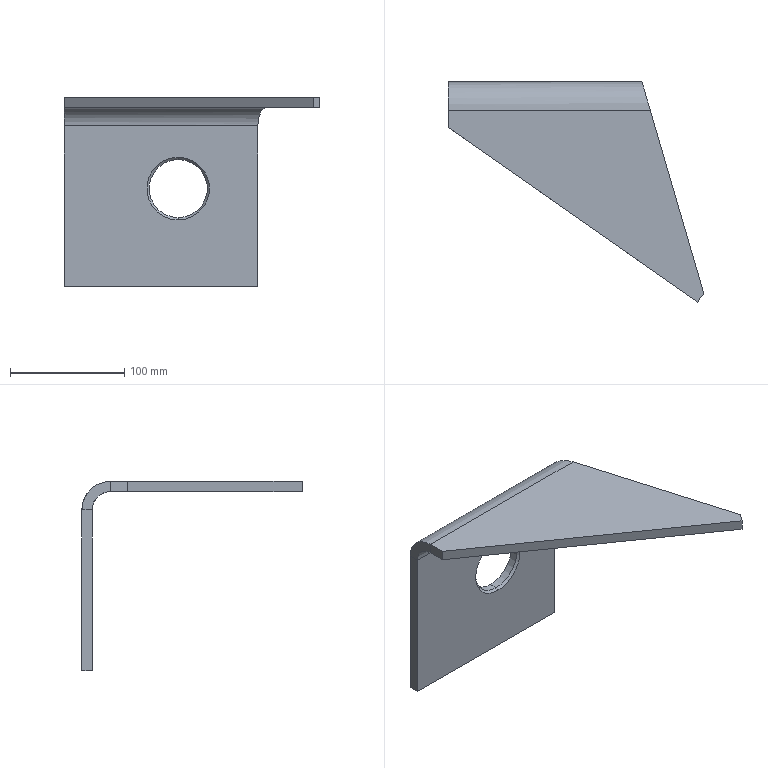Part | SolidWorks | features ICE 2, Chamfer 1, FlatPattern 1, SMBaseFlange 1, SheetMetal 1 | 1 solid | 19 faces | box 224.289 x 193.117 x 166 mm | volume 401605 mm3 | plane 12 | cylinder 4 | cone 2 | spline 1 | commonest cylinder face diameters 51 x2 32 x1 50 x1
STEP:
#1=CARTESIAN_POINT('',(100.,-7.,111.5));
#2=VERTEX_POINT('',#1);
#3=CARTESIAN_POINT('',(100.,-7.,60.5));
#4=VERTEX_POINT('',#3);
#5=CARTESIAN_POINT('',(100.,-7.,86.));
#6=DIRECTION('',(0.,-1.,0.));
#7=DIRECTION('',(0.,0.,-1.));
#8=AXIS2_PLACEMENT_3D('',#5,#6,#7);
#9=CIRCLE('',#8,25.5);
#10=EDGE_CURVE('',#2,#4,#9,.T.);
#11=ORIENTED_EDGE('',*,*,#10,.F.);
#12=CARTESIAN_POINT('',(100.,-9.,113.5));
#13=VERTEX_POINT('',#12);
#14=CARTESIAN_POINT('',(100.,-7.,111.5));
#15=DIRECTION('',(0.,-0.7071,0.7071));
#16=VECTOR('',#15,1000.);
#17=LINE('',#14,#16);
#18=EDGE_CURVE('',#2,#13,#17,.T.);
#19=ORIENTED_EDGE('',*,*,#18,.T.);
#20=CARTESIAN_POINT('',(100.,-9.,58.5));
#21=VERTEX_POINT('',#20);
#22=CARTESIAN_POINT('',(100.,-9.,86.));
#23=DIRECTION('',(0.,1.,0.));
#24=DIRECTION('',(0.,0.,-1.));
#25=AXIS2_PLACEMENT_3D('',#22,#23,#24);
#26=CIRCLE('',#25,27.5);
#27=EDGE_CURVE('',#21,#13,#26,.T.);
#28=ORIENTED_EDGE('',*,*,#27,.F.);
#29=CARTESIAN_POINT('',(100.,-7.,60.5));
#30=DIRECTION('',(0.,-0.7071,-0.7071));
#31=VECTOR('',#30,1000.);
#32=LINE('',#29,#31);
#33=EDGE_CURVE('',#4,#21,#32,.T.);
#34=ORIENTED_EDGE('',*,*,#33,.F.);
#35=EDGE_LOOP('',(#11,#19,#28,#34));
#36=FACE_OUTER_BOUND('',#35,.T.);
#37=CARTESIAN_POINT('',(100.,-7.,86.));
#38=DIRECTION('',(0.,-1.,0.));
#39=DIRECTION('',(0.,0.,-1.));
#40=AXIS2_PLACEMENT_3D('',#37,#38,#39);
#41=CONICAL_SURFACE('',#40,25.5,0.7854);
#42=ADVANCED_FACE('',(#36),#41,.F.);
#43=ORIENTED_EDGE('',*,*,#10,.T.);
#44=CARTESIAN_POINT('',(100.,0.,60.5));
#45=VERTEX_POINT('',#44);
#46=CARTESIAN_POINT('',(100.,-193.117,60.5));
#47=DIRECTION('',(0.,1.,0.));
#48=VECTOR('',#47,1000.);
#49=LINE('',#46,#48);
#50=EDGE_CURVE('',#4,#45,#49,.T.);
#51=ORIENTED_EDGE('',*,*,#50,.T.);
#52=CARTESIAN_POINT('',(100.,0.,111.5));
#53=VERTEX_POINT('',#52);
#54=CARTESIAN_POINT('',(100.,0.,86.));
#55=DIRECTION('',(0.,1.,0.));
#56=DIRECTION('',(0.,0.,1.));
#57=AXIS2_PLACEMENT_3D('',#54,#55,#56);
#58=CIRCLE('',#57,25.5);
#59=EDGE_CURVE('',#45,#53,#58,.T.);
#60=ORIENTED_EDGE('',*,*,#59,.T.);
#61=CARTESIAN_POINT('',(100.,-193.117,111.5));
#62=DIRECTION('',(0.,1.,0.));
#63=VECTOR('',#62,1000.);
#64=LINE('',#61,#63);
#65=EDGE_CURVE('',#2,#53,#64,.T.);
#66=ORIENTED_EDGE('',*,*,#65,.F.);
#67=EDGE_LOOP('',(#43,#51,#60,#66));
#68=FACE_OUTER_BOUND('',#67,.T.);
#69=CARTESIAN_POINT('',(100.,-193.117,86.));
#70=DIRECTION('',(0.,1.,0.));
#71=DIRECTION('',(0.,0.,1.));
#72=AXIS2_PLACEMENT_3D('',#69,#70,#71);
#73=CYLINDRICAL_SURFACE('',#72,25.5);
#74=ADVANCED_FACE('',(#68),#73,.F.);
#75=CARTESIAN_POINT('',(0.,-25.,157.));
#76=VERTEX_POINT('',#75);
#77=CARTESIAN_POINT('',(0.,-40.,157.));
#78=VERTEX_POINT('',#77);
#79=CARTESIAN_POINT('',(0.,0.,157.));
#80=DIRECTION('',(0.,-1.,0.));
#81=VECTOR('',#80,1000.);
#82=LINE('',#79,#81);
#83=EDGE_CURVE('',#76,#78,#82,.T.);
#84=ORIENTED_EDGE('',*,*,#83,.T.);
#85=CARTESIAN_POINT('',(0.,-40.,166.));
#86=VERTEX_POINT('',#85);
#87=CARTESIAN_POINT('',(0.,-40.,157.));
#88=DIRECTION('',(0.,0.,1.));
#89=VECTOR('',#88,1000.);
#90=LINE('',#87,#89);
#91=EDGE_CURVE('',#78,#86,#90,.T.);
#92=ORIENTED_EDGE('',*,*,#91,.T.);
#93=CARTESIAN_POINT('',(0.,-25.,166.));
#94=VERTEX_POINT('',#93);
#95=CARTESIAN_POINT('',(0.,0.,166.));
#96=DIRECTION('',(0.,-1.,0.));
#97=VECTOR('',#96,1000.);
#98=LINE('',#95,#97);
#99=EDGE_CURVE('',#94,#86,#98,.T.);
#100=ORIENTED_EDGE('',*,*,#99,.F.);
#101=CARTESIAN_POINT('',(0.,-25.,166.));
#102=DIRECTION('',(0.,0.,-1.));
#103=VECTOR('',#102,1000.);
#104=LINE('',#101,#103);
#105=EDGE_CURVE('',#94,#76,#104,.T.);
#106=ORIENTED_EDGE('',*,*,#105,.T.);
#107=EDGE_LOOP('',(#84,#92,#100,#106));
#108=FACE_OUTER_BOUND('',#107,.T.);
#109=CARTESIAN_POINT('',(0.,-9.,141.));
#110=DIRECTION('',(-1.,0.,0.));
#111=DIRECTION('',(0.,0.,1.));
#112=AXIS2_PLACEMENT_3D('',#109,#110,#111);
#113=PLANE('',#112);
#114=ADVANCED_FACE('',(#108),#113,.T.);
#115=CARTESIAN_POINT('',(218.67,-193.117,166.));
#116=VERTEX_POINT('',#115);
#117=CARTESIAN_POINT('',(134.53,-134.201,166.));
#118=DIRECTION('',(0.8191,-0.5736,0.));
#119=VECTOR('',#118,1000.);
#120=LINE('',#117,#119);
#121=EDGE_CURVE('',#86,#116,#120,.T.);
#122=ORIENTED_EDGE('',*,*,#121,.T.);
#123=CARTESIAN_POINT('',(224.289,-185.603,166.));
#124=VERTEX_POINT('',#123);
#125=CARTESIAN_POINT('',(314.815,-64.545,166.));
#126=DIRECTION('',(0.5989,0.8008,0.));
#127=VECTOR('',#126,1000.);
#128=LINE('',#125,#127);
#129=EDGE_CURVE('',#116,#124,#128,.T.);
#130=ORIENTED_EDGE('',*,*,#129,.T.);
#131=CARTESIAN_POINT('',(177.312,-25.,166.));
#132=VERTEX_POINT('',#131);
#133=CARTESIAN_POINT('',(174.611,-15.763,166.));
#134=DIRECTION('',(-0.2807,0.9598,0.));
#135=VECTOR('',#134,1000.);
#136=LINE('',#133,#135);
#137=EDGE_CURVE('',#124,#132,#136,.T.);
#138=ORIENTED_EDGE('',*,*,#137,.T.);
#139=CARTESIAN_POINT('',(228.5,-25.,166.));
#140=DIRECTION('',(-1.,0.,0.));
#141=VECTOR('',#140,1000.);
#142=LINE('',#139,#141);
#143=EDGE_CURVE('',#132,#94,#142,.T.);
#144=ORIENTED_EDGE('',*,*,#143,.T.);
#145=ORIENTED_EDGE('',*,*,#99,.T.);
#146=EDGE_LOOP('',(#122,#130,#138,#144,#145));
#147=FACE_OUTER_BOUND('',#146,.T.);
#148=CARTESIAN_POINT('',(228.5,0.,166.));
#149=DIRECTION('',(0.,0.,-1.));
#150=DIRECTION('',(-1.,0.,0.));
#151=AXIS2_PLACEMENT_3D('',#148,#149,#150);
#152=PLANE('',#151);
#153=ADVANCED_FACE('',(#147),#152,.F.);
#154=CARTESIAN_POINT('',(218.67,-193.117,157.));
#155=VERTEX_POINT('',#154);
#156=CARTESIAN_POINT('',(224.289,-185.603,157.));
#157=VERTEX_POINT('',#156);
#158=CARTESIAN_POINT('',(314.815,-64.545,157.));
#159=DIRECTION('',(0.5989,0.8008,0.));
#160=VECTOR('',#159,1000.);
#161=LINE('',#158,#160);
#162=EDGE_CURVE('',#155,#157,#161,.T.);
#163=ORIENTED_EDGE('',*,*,#162,.F.);
#164=CARTESIAN_POINT('',(134.53,-134.201,157.));
#165=DIRECTION('',(0.8191,-0.5736,0.));
#166=VECTOR('',#165,1000.);
#167=LINE('',#164,#166);
#168=EDGE_CURVE('',#78,#155,#167,.T.);
#169=ORIENTED_EDGE('',*,*,#168,.F.);
#170=ORIENTED_EDGE('',*,*,#83,.F.);
#171=CARTESIAN_POINT('',(177.312,-25.,157.));
#172=VERTEX_POINT('',#171);
#173=CARTESIAN_POINT('',(228.5,-25.,157.));
#174=DIRECTION('',(-1.,0.,0.));
#175=VECTOR('',#174,1000.);
#176=LINE('',#173,#175);
#177=EDGE_CURVE('',#172,#76,#176,.T.);
#178=ORIENTED_EDGE('',*,*,#177,.F.);
#179=CARTESIAN_POINT('',(174.611,-15.763,157.));
#180=DIRECTION('',(-0.2807,0.9598,0.));
#181=VECTOR('',#180,1000.);
#182=LINE('',#179,#181);
#183=EDGE_CURVE('',#157,#172,#182,.T.);
#184=ORIENTED_EDGE('',*,*,#183,.F.);
#185=EDGE_LOOP('',(#163,#169,#170,#178,#184));
#186=FACE_OUTER_BOUND('',#185,.T.);
#187=CARTESIAN_POINT('',(228.5,0.,157.));
#188=DIRECTION('',(0.,0.,-1.));
#189=DIRECTION('',(-1.,0.,0.));
#190=AXIS2_PLACEMENT_3D('',#187,#188,#189);
#191=PLANE('',#190);
#192=ADVANCED_FACE('',(#186),#191,.T.);
#193=CARTESIAN_POINT('',(170.,-9.,141.));
#194=VERTEX_POINT('',#193);
#195=CARTESIAN_POINT('',(0.,-9.,141.));
#196=VERTEX_POINT('',#195);
#197=CARTESIAN_POINT('',(228.5,-9.,141.));
#198=DIRECTION('',(-1.,0.,0.));
#199=VECTOR('',#198,1000.);
#200=LINE('',#197,#199);
#201=EDGE_CURVE('',#194,#196,#200,.T.);
#202=ORIENTED_EDGE('',*,*,#201,.F.);
#203=CARTESIAN_POINT('',(177.312,-25.,157.));
#204=CARTESIAN_POINT('',(173.029,-15.627,157.));
#205=CARTESIAN_POINT('',(170.,-9.,150.373));
#206=CARTESIAN_POINT('',(170.,-9.,141.));
#207=(BOUNDED_CURVE()B_SPLINE_CURVE(3,(#203,#204,#205,#206),.UNSPECIFIED.,.F.,.T.)B_SPLINE_CURVE_WITH_KNOTS((4,4),(4.712,6.283),.UNSPECIFIED.)CURVE()GEOMETRIC_REPRESENTATION_ITEM()RATIONAL_B_SPLINE_CURVE((1.,0.8047,0.8047,1.))REPRESENTATION_ITEM(''));
#208=EDGE_CURVE('',#172,#194,#207,.T.);
#209=ORIENTED_EDGE('',*,*,#208,.F.);
#210=ORIENTED_EDGE('',*,*,#177,.T.);
#211=CARTESIAN_POINT('',(0.,-25.,141.));
#212=DIRECTION('',(1.,0.,0.));
#213=DIRECTION('',(0.,0.,-1.));
#214=AXIS2_PLACEMENT_3D('',#211,#212,#213);
#215=CIRCLE('',#214,16.);
#216=EDGE_CURVE('',#196,#76,#215,.T.);
#217=ORIENTED_EDGE('',*,*,#216,.F.);
#218=EDGE_LOOP('',(#202,#209,#210,#217));
#219=FACE_OUTER_BOUND('',#218,.T.);
#220=CARTESIAN_POINT('',(228.5,-25.,141.));
#221=DIRECTION('',(-1.,0.,0.));
#222=DIRECTION('',(0.,0.,1.));
#223=AXIS2_PLACEMENT_3D('',#220,#221,#222);
#224=CYLINDRICAL_SURFACE('',#223,16.);
#225=ADVANCED_FACE('',(#219),#224,.F.);
#226=ORIENTED_EDGE('',*,*,#27,.T.);
#227=CARTESIAN_POINT('',(100.,-9.,86.));
#228=DIRECTION('',(0.,1.,0.));
#229=DIRECTION('',(0.,0.,-1.));
#230=AXIS2_PLACEMENT_3D('',#227,#228,#229);
#231=CIRCLE('',#230,27.5);
#232=EDGE_CURVE('',#13,#21,#231,.T.);
#233=ORIENTED_EDGE('',*,*,#232,.T.);
#234=EDGE_LOOP('',(#226,#233));
#235=FACE_BOUND('',#234,.T.);
#236=CARTESIAN_POINT('',(170.,-9.,0.));
#237=VERTEX_POINT('',#236);
#238=CARTESIAN_POINT('',(0.,-9.,0.));
#239=VERTEX_POINT('',#238);
#240=CARTESIAN_POINT('',(228.5,-9.,0.));
#241=DIRECTION('',(-1.,0.,0.));
#242=VECTOR('',#241,1000.);
#243=LINE('',#240,#242);
#244=EDGE_CURVE('',#237,#239,#243,.T.);
#245=ORIENTED_EDGE('',*,*,#244,.F.);
#246=CARTESIAN_POINT('',(170.,-9.,0.));
#247=DIRECTION('',(0.,0.,1.));
#248=VECTOR('',#247,1000.);
#249=LINE('',#246,#248);
#250=EDGE_CURVE('',#237,#194,#249,.T.);
#251=ORIENTED_EDGE('',*,*,#250,.T.);
#252=ORIENTED_EDGE('',*,*,#201,.T.);
#253=CARTESIAN_POINT('',(0.,-9.,0.));
#254=DIRECTION('',(0.,0.,1.));
#255=VECTOR('',#254,1000.);
#256=LINE('',#253,#255);
#257=EDGE_CURVE('',#239,#196,#256,.T.);
#258=ORIENTED_EDGE('',*,*,#257,.F.);
#259=EDGE_LOOP('',(#245,#251,#252,#258));
#260=FACE_OUTER_BOUND('',#259,.T.);
#261=CARTESIAN_POINT('',(228.5,-9.,0.));
#262=DIRECTION('',(0.,-1.,0.));
#263=DIRECTION('',(0.,0.,-1.));
#264=AXIS2_PLACEMENT_3D('',#261,#262,#263);
#265=PLANE('',#264);
#266=ADVANCED_FACE('',(#235,#260),#265,.T.);
#267=CARTESIAN_POINT('',(170.,0.,0.));
#268=VERTEX_POINT('',#267);
#269=CARTESIAN_POINT('',(0.,0.,0.));
#270=VERTEX_POINT('',#269);
#271=CARTESIAN_POINT('',(228.5,0.,0.));
#272=DIRECTION('',(-1.,0.,0.));
#273=VECTOR('',#272,1000.);
#274=LINE('',#271,#273);
#275=EDGE_CURVE('',#268,#270,#274,.T.);
#276=ORIENTED_EDGE('',*,*,#275,.F.);
#277=CARTESIAN_POINT('',(170.,0.,0.));
#278=DIRECTION('',(0.,-1.,0.));
#279=VECTOR('',#278,1000.);
#280=LINE('',#277,#279);
#281=EDGE_CURVE('',#268,#237,#280,.T.);
#282=ORIENTED_EDGE('',*,*,#281,.T.);
#283=ORIENTED_EDGE('',*,*,#244,.T.);
#284=CARTESIAN_POINT('',(0.,0.,0.));
#285=DIRECTION('',(0.,-1.,0.));
#286=VECTOR('',#285,1000.);
#287=LINE('',#284,#286);
#288=EDGE_CURVE('',#270,#239,#287,.T.);
#289=ORIENTED_EDGE('',*,*,#288,.F.);
#290=EDGE_LOOP('',(#276,#282,#283,#289));
#291=FACE_OUTER_BOUND('',#290,.T.);
#292=CARTESIAN_POINT('',(228.5,0.,0.));
#293=DIRECTION('',(0.,0.,-1.));
#294=DIRECTION('',(-1.,0.,0.));
#295=AXIS2_PLACEMENT_3D('',#292,#293,#294);
#296=PLANE('',#295);
#297=ADVANCED_FACE('',(#291),#296,.T.);
#298=CARTESIAN_POINT('',(100.,0.,86.));
#299=DIRECTION('',(0.,1.,0.));
#300=DIRECTION('',(0.,0.,1.));
#301=AXIS2_PLACEMENT_3D('',#298,#299,#300);
#302=CIRCLE('',#301,25.5);
#303=EDGE_CURVE('',#53,#45,#302,.T.);
#304=ORIENTED_EDGE('',*,*,#303,.F.);
#305=ORIENTED_EDGE('',*,*,#59,.F.);
#306=EDGE_LOOP('',(#304,#305));
#307=FACE_BOUND('',#306,.T.);
#308=CARTESIAN_POINT('',(170.,0.,141.));
#309=VERTEX_POINT('',#308);
#310=CARTESIAN_POINT('',(170.,0.,0.));
#311=DIRECTION('',(0.,0.,1.));
#312=VECTOR('',#311,1000.);
#313=LINE('',#310,#312);
#314=EDGE_CURVE('',#268,#309,#313,.T.);
#315=ORIENTED_EDGE('',*,*,#314,.F.);
#316=ORIENTED_EDGE('',*,*,#275,.T.);
#317=CARTESIAN_POINT('',(0.,0.,141.));
#318=VERTEX_POINT('',#317);
#319=CARTESIAN_POINT('',(0.,0.,0.));
#320=DIRECTION('',(0.,0.,1.));
#321=VECTOR('',#320,1000.);
#322=LINE('',#319,#321);
#323=EDGE_CURVE('',#270,#318,#322,.T.);
#324=ORIENTED_EDGE('',*,*,#323,.T.);
#325=CARTESIAN_POINT('',(228.5,0.,141.));
#326=DIRECTION('',(-1.,0.,0.));
#327=VECTOR('',#326,1000.);
#328=LINE('',#325,#327);
#329=EDGE_CURVE('',#309,#318,#328,.T.);
#330=ORIENTED_EDGE('',*,*,#329,.F.);
#331=EDGE_LOOP('',(#315,#316,#324,#330));
#332=FACE_OUTER_BOUND('',#331,.T.);
#333=CARTESIAN_POINT('',(228.5,0.,0.));
#334=DIRECTION('',(0.,-1.,0.));
#335=DIRECTION('',(0.,0.,-1.));
#336=AXIS2_PLACEMENT_3D('',#333,#334,#335);
#337=PLANE('',#336);
#338=ADVANCED_FACE('',(#307,#332),#337,.F.);
#339=CARTESIAN_POINT('',(177.312,-25.,166.));
#340=CARTESIAN_POINT('',(173.029,-10.355,166.));
#341=CARTESIAN_POINT('',(170.,0.,155.645));
#342=CARTESIAN_POINT('',(170.,0.,141.));
#343=(BOUNDED_CURVE()B_SPLINE_CURVE(3,(#339,#340,#341,#342),.UNSPECIFIED.,.F.,.T.)B_SPLINE_CURVE_WITH_KNOTS((4,4),(4.712,6.283),.UNSPECIFIED.)CURVE()GEOMETRIC_REPRESENTATION_ITEM()RATIONAL_B_SPLINE_CURVE((1.,0.8047,0.8047,1.))REPRESENTATION_ITEM(''));
#344=EDGE_CURVE('',#132,#309,#343,.T.);
#345=ORIENTED_EDGE('',*,*,#344,.T.);
#346=ORIENTED_EDGE('',*,*,#329,.T.);
#347=CARTESIAN_POINT('',(0.,-25.,141.));
#348=DIRECTION('',(1.,0.,0.));
#349=DIRECTION('',(0.,0.,1.));
#350=AXIS2_PLACEMENT_3D('',#347,#348,#349);
#351=CIRCLE('',#350,25.);
#352=EDGE_CURVE('',#318,#94,#351,.T.);
#353=ORIENTED_EDGE('',*,*,#352,.T.);
#354=ORIENTED_EDGE('',*,*,#143,.F.);
#355=EDGE_LOOP('',(#345,#346,#353,#354));
#356=FACE_OUTER_BOUND('',#355,.T.);
#357=CARTESIAN_POINT('',(228.5,-25.,141.));
#358=DIRECTION('',(-1.,0.,0.));
#359=DIRECTION('',(0.,0.,1.));
#360=AXIS2_PLACEMENT_3D('',#357,#358,#359);
#361=CYLINDRICAL_SURFACE('',#360,25.);
#362=ADVANCED_FACE('',(#356),#361,.T.);
#363=ORIENTED_EDGE('',*,*,#105,.F.);
#364=ORIENTED_EDGE('',*,*,#352,.F.);
#365=CARTESIAN_POINT('',(0.,-9.,141.));
#366=DIRECTION('',(0.,1.,0.));
#367=VECTOR('',#366,1000.);
#368=LINE('',#365,#367);
#369=EDGE_CURVE('',#196,#318,#368,.T.);
#370=ORIENTED_EDGE('',*,*,#369,.F.);
#371=ORIENTED_EDGE('',*,*,#216,.T.);
#372=EDGE_LOOP('',(#363,#364,#370,#371));
#373=FACE_OUTER_BOUND('',#372,.T.);
#374=CARTESIAN_POINT('',(0.,-25.,166.));
#375=DIRECTION('',(-1.,0.,0.));
#376=DIRECTION('',(0.,0.,1.));
#377=AXIS2_PLACEMENT_3D('',#374,#375,#376);
#378=PLANE('',#377);
#379=ADVANCED_FACE('',(#373),#378,.T.);
#380=ORIENTED_EDGE('',*,*,#257,.T.);
#381=ORIENTED_EDGE('',*,*,#369,.T.);
#382=ORIENTED_EDGE('',*,*,#323,.F.);
#383=ORIENTED_EDGE('',*,*,#288,.T.);
#384=EDGE_LOOP('',(#380,#381,#382,#383));
#385=FACE_OUTER_BOUND('',#384,.T.);
#386=CARTESIAN_POINT('',(0.,-25.,141.));
#387=DIRECTION('',(1.,0.,0.));
#388=DIRECTION('',(0.,0.,-1.));
#389=AXIS2_PLACEMENT_3D('',#386,#387,#388);
#390=PLANE('',#389);
#391=ADVANCED_FACE('',(#385),#390,.F.);
#392=ORIENTED_EDGE('',*,*,#91,.F.);
#393=ORIENTED_EDGE('',*,*,#168,.T.);
#394=CARTESIAN_POINT('',(218.67,-193.117,157.));
#395=DIRECTION('',(0.,0.,1.));
#396=VECTOR('',#395,1000.);
#397=LINE('',#394,#396);
#398=EDGE_CURVE('',#155,#116,#397,.T.);
#399=ORIENTED_EDGE('',*,*,#398,.T.);
#400=ORIENTED_EDGE('',*,*,#121,.F.);
#401=EDGE_LOOP('',(#392,#393,#399,#400));
#402=FACE_OUTER_BOUND('',#401,.T.);
#403=CARTESIAN_POINT('',(134.53,-134.201,157.));
#404=DIRECTION('',(0.5736,0.8191,0.));
#405=DIRECTION('',(0.8191,-0.5736,0.));
#406=AXIS2_PLACEMENT_3D('',#403,#404,#405);
#407=PLANE('',#406);
#408=ADVANCED_FACE('',(#402),#407,.F.);
#409=ORIENTED_EDGE('',*,*,#398,.F.);
#410=ORIENTED_EDGE('',*,*,#162,.T.);
#411=CARTESIAN_POINT('',(224.289,-185.603,157.));
#412=DIRECTION('',(0.,0.,1.));
#413=VECTOR('',#412,1000.);
#414=LINE('',#411,#413);
#415=EDGE_CURVE('',#157,#124,#414,.T.);
#416=ORIENTED_EDGE('',*,*,#415,.T.);
#417=ORIENTED_EDGE('',*,*,#129,.F.);
#418=EDGE_LOOP('',(#409,#410,#416,#417));
#419=FACE_OUTER_BOUND('',#418,.T.);
#420=CARTESIAN_POINT('',(314.815,-64.545,157.));
#421=DIRECTION('',(-0.8008,0.5989,0.));
#422=DIRECTION('',(0.5989,0.8008,0.));
#423=AXIS2_PLACEMENT_3D('',#420,#421,#422);
#424=PLANE('',#423);
#425=ADVANCED_FACE('',(#419),#424,.F.);
#426=ORIENTED_EDGE('',*,*,#183,.T.);
#427=CARTESIAN_POINT('',(177.312,-25.,157.));
#428=DIRECTION('',(0.,0.,1.));
#429=VECTOR('',#428,1000.);
#430=LINE('',#427,#429);
#431=EDGE_CURVE('',#172,#132,#430,.T.);
#432=ORIENTED_EDGE('',*,*,#431,.T.);
#433=ORIENTED_EDGE('',*,*,#137,.F.);
#434=ORIENTED_EDGE('',*,*,#415,.F.);
#435=EDGE_LOOP('',(#426,#432,#433,#434));
#436=FACE_OUTER_BOUND('',#435,.T.);
#437=CARTESIAN_POINT('',(174.611,-15.763,157.));
#438=DIRECTION('',(-0.9598,-0.2807,0.));
#439=DIRECTION('',(-0.2807,0.9598,0.));
#440=AXIS2_PLACEMENT_3D('',#437,#438,#439);
#441=PLANE('',#440);
#442=ADVANCED_FACE('',(#436),#441,.F.);
#443=ORIENTED_EDGE('',*,*,#281,.F.);
#444=ORIENTED_EDGE('',*,*,#314,.T.);
#445=CARTESIAN_POINT('',(170.,0.,141.));
#446=DIRECTION('',(0.,-1.,0.));
#447=VECTOR('',#446,1000.);
#448=LINE('',#445,#447);
#449=EDGE_CURVE('',#309,#194,#448,.T.);
#450=ORIENTED_EDGE('',*,*,#449,.T.);
#451=ORIENTED_EDGE('',*,*,#250,.F.);
#452=EDGE_LOOP('',(#443,#444,#450,#451));
#453=FACE_OUTER_BOUND('',#452,.T.);
#454=CARTESIAN_POINT('',(170.,0.,0.));
#455=DIRECTION('',(1.,0.,0.));
#456=DIRECTION('',(0.,0.,1.));
#457=AXIS2_PLACEMENT_3D('',#454,#455,#456);
#458=PLANE('',#457);
#459=ADVANCED_FACE('',(#453),#458,.T.);
#460=ORIENTED_EDGE('',*,*,#449,.F.);
#461=ORIENTED_EDGE('',*,*,#344,.F.);
#462=ORIENTED_EDGE('',*,*,#431,.F.);
#463=ORIENTED_EDGE('',*,*,#208,.T.);
#464=EDGE_LOOP('',(#460,#461,#462,#463));
#465=FACE_OUTER_BOUND('',#464,.T.);
#466=CARTESIAN_POINT('',(170.,-9.,141.));
#467=CARTESIAN_POINT('',(170.,-6.,141.));
#468=CARTESIAN_POINT('',(170.,-3.,141.));
#469=CARTESIAN_POINT('',(170.,0.,141.));
#470=CARTESIAN_POINT('',(170.,-9.,109.));
#471=CARTESIAN_POINT('',(170.,-6.,103.));
#472=CARTESIAN_POINT('',(170.,-3.,97.));
#473=CARTESIAN_POINT('',(170.,0.,91.));
#474=CARTESIAN_POINT('',(184.625,-41.,109.));
#475=CARTESIAN_POINT('',(184.625,-44.,103.));
#476=CARTESIAN_POINT('',(184.625,-47.,97.));
#477=CARTESIAN_POINT('',(184.625,-50.,91.));
#478=CARTESIAN_POINT('',(184.625,-41.,141.));
#479=CARTESIAN_POINT('',(184.625,-44.,141.));
#480=CARTESIAN_POINT('',(184.625,-47.,141.));
#481=CARTESIAN_POINT('',(184.625,-50.,141.));
#482=CARTESIAN_POINT('',(184.625,-41.,173.));
#483=CARTESIAN_POINT('',(184.625,-44.,179.));
#484=CARTESIAN_POINT('',(184.625,-47.,185.));
#485=CARTESIAN_POINT('',(184.625,-50.,191.));
#486=CARTESIAN_POINT('',(170.,-9.,173.));
#487=CARTESIAN_POINT('',(170.,-6.,179.));
#488=CARTESIAN_POINT('',(170.,-3.,185.));
#489=CARTESIAN_POINT('',(170.,0.,191.));
#490=CARTESIAN_POINT('',(170.,-9.,141.));
#491=CARTESIAN_POINT('',(170.,-6.,141.));
#492=CARTESIAN_POINT('',(170.,-3.,141.));
#493=CARTESIAN_POINT('',(170.,0.,141.));
#494=(BOUNDED_SURFACE()B_SPLINE_SURFACE(3,3,((#466,#467,#468,#469),(#470,#471,#472,#473),(#474,#475,#476,#477),(#478,#479,#480,#481),(#482,#483,#484,#485),(#486,#487,#488,#489),(#490,#491,#492,#493)),.UNSPECIFIED.,.T.,.F.,.T.)B_SPLINE_SURFACE_WITH_KNOTS((4,3,4),(4,4),(0.,0.5,1.),(0.,1.),.UNSPECIFIED.)GEOMETRIC_REPRESENTATION_ITEM()RATIONAL_B_SPLINE_SURFACE(((1.,1.,1.,1.),(0.3333,0.3333,0.3333,0.3333),(0.3333,0.3333,0.3333,0.3333),(1.,1.,1.,1.),(0.3333,0.3333,0.3333,0.3333),(0.3333,0.3333,0.3333,0.3333),(1.,1.,1.,1.)))REPRESENTATION_ITEM('')SURFACE());
#495=ADVANCED_FACE('',(#465),#494,.T.);
#496=ORIENTED_EDGE('',*,*,#50,.F.);
#497=CARTESIAN_POINT('',(100.,-7.,86.));
#498=DIRECTION('',(0.,-1.,0.));
#499=DIRECTION('',(0.,0.,-1.));
#500=AXIS2_PLACEMENT_3D('',#497,#498,#499);
#501=CIRCLE('',#500,25.5);
#502=EDGE_CURVE('',#4,#2,#501,.T.);
#503=ORIENTED_EDGE('',*,*,#502,.T.);
#504=ORIENTED_EDGE('',*,*,#65,.T.);
#505=ORIENTED_EDGE('',*,*,#303,.T.);
#506=EDGE_LOOP('',(#496,#503,#504,#505));
#507=FACE_OUTER_BOUND('',#506,.T.);
#508=CARTESIAN_POINT('',(100.,-193.117,86.));
#509=DIRECTION('',(0.,1.,0.));
#510=DIRECTION('',(0.,0.,1.));
#511=AXIS2_PLACEMENT_3D('',#508,#509,#510);
#512=CYLINDRICAL_SURFACE('',#511,25.5);
#513=ADVANCED_FACE('',(#507),#512,.F.);
#514=ORIENTED_EDGE('',*,*,#18,.F.);
#515=ORIENTED_EDGE('',*,*,#502,.F.);
#516=ORIENTED_EDGE('',*,*,#33,.T.);
#517=ORIENTED_EDGE('',*,*,#232,.F.);
#518=EDGE_LOOP('',(#514,#515,#516,#517));
#519=FACE_OUTER_BOUND('',#518,.T.);
#520=CARTESIAN_POINT('',(100.,-7.,86.));
#521=DIRECTION('',(0.,-1.,0.));
#522=DIRECTION('',(0.,0.,-1.));
#523=AXIS2_PLACEMENT_3D('',#520,#521,#522);
#524=CONICAL_SURFACE('',#523,25.5,0.7854);
#525=ADVANCED_FACE('',(#519),#524,.F.);
#526=CLOSED_SHELL('',(#42,#74,#114,#153,#192,#225,#266,#297,#338,#362,#379,#391,#408,#425,#442,#459,#495,#513,#525));
#527=MANIFOLD_SOLID_BREP('',#526);
#528=CARTESIAN_POINT('',(0.,0.,0.));
#529=DIRECTION('',(0.,0.,1.));
#530=DIRECTION('',(1.,0.,0.));
#531=AXIS2_PLACEMENT_3D('',#528,#529,#530);
#532=(LENGTH_UNIT()NAMED_UNIT(*)SI_UNIT(.MILLI.,.METRE.));
#533=UNCERTAINTY_MEASURE_WITH_UNIT(LENGTH_MEASURE(0.00001),#532,'','');
#534=(NAMED_UNIT(*)PLANE_ANGLE_UNIT()SI_UNIT($,.RADIAN.));
#535=(NAMED_UNIT(*)SI_UNIT($,.STERADIAN.)SOLID_ANGLE_UNIT());
#536=(GEOMETRIC_REPRESENTATION_CONTEXT(3)GLOBAL_UNCERTAINTY_ASSIGNED_CONTEXT((#533))GLOBAL_UNIT_ASSIGNED_CONTEXT((#532,#534,#535))REPRESENTATION_CONTEXT('',''));
#537=ADVANCED_BREP_SHAPE_REPRESENTATION('',(#527,#531),#536);